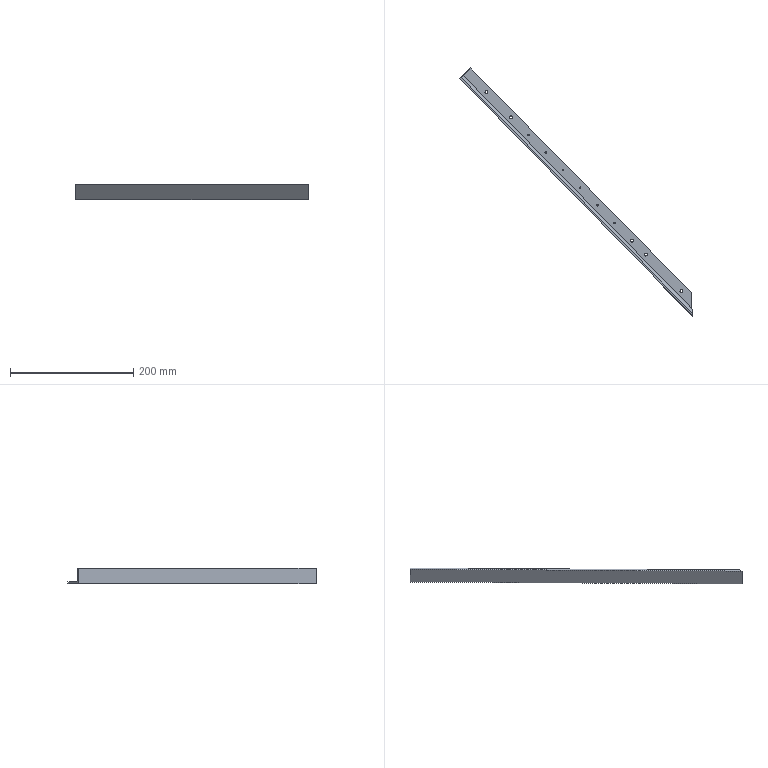Part | NX | features MG0301 nose pivot 24(right) 2 | 1 solid | 20 faces | box 376.796 x 401.943 x 25.4 mm | volume 82340 mm3 | cylinder 12 | plane 8 | commonest cylinder face diameters 2.4 x6 4.763 x5 9.525 x1
STEP:
#1=CARTESIAN_POINT('',(-216.606,-252.536,3.175));
#2=VERTEX_POINT('',#1);
#3=CARTESIAN_POINT('',(-217.446,-251.679,3.175));
#4=DIRECTION('',(0.,0.,1.));
#5=DIRECTION('',(0.7002,-0.7139,0.));
#6=AXIS2_PLACEMENT_3D('',#3,#4,#5);
#7=CIRCLE('',#6,1.2);
#8=EDGE_CURVE('',#2,#2,#7,.T.);
#9=ORIENTED_EDGE('',*,*,#8,.F.);
#10=EDGE_LOOP('',(#9));
#11=FACE_BOUND('',#10,.T.);
#12=CARTESIAN_POINT('',(-160.587,-309.649,3.175));
#13=VERTEX_POINT('',#12);
#14=CARTESIAN_POINT('',(-161.428,-308.792,3.175));
#15=DIRECTION('',(0.,0.,1.));
#16=DIRECTION('',(0.7002,-0.7139,0.));
#17=AXIS2_PLACEMENT_3D('',#14,#15,#16);
#18=CIRCLE('',#17,1.2);
#19=EDGE_CURVE('',#13,#13,#18,.T.);
#20=ORIENTED_EDGE('',*,*,#19,.F.);
#21=EDGE_LOOP('',(#20));
#22=FACE_BOUND('',#21,.T.);
#23=CARTESIAN_POINT('',(-104.569,-366.762,3.175));
#24=VERTEX_POINT('',#23);
#25=CARTESIAN_POINT('',(-105.409,-365.905,3.175));
#26=DIRECTION('',(0.,0.,1.));
#27=DIRECTION('',(0.7002,-0.7139,0.));
#28=AXIS2_PLACEMENT_3D('',#25,#26,#27);
#29=CIRCLE('',#28,1.2);
#30=EDGE_CURVE('',#24,#24,#29,.T.);
#31=ORIENTED_EDGE('',*,*,#30,.F.);
#32=EDGE_LOOP('',(#31));
#33=FACE_BOUND('',#32,.T.);
#34=CARTESIAN_POINT('',(-271.084,-194.566,3.175));
#35=VERTEX_POINT('',#34);
#36=CARTESIAN_POINT('',(-273.465,-194.566,3.175));
#37=DIRECTION('',(0.,0.,1.));
#38=DIRECTION('',(1.,0.,0.));
#39=AXIS2_PLACEMENT_3D('',#36,#37,#38);
#40=CIRCLE('',#39,2.381);
#41=EDGE_CURVE('',#35,#35,#40,.T.);
#42=ORIENTED_EDGE('',*,*,#41,.F.);
#43=EDGE_LOOP('',(#42));
#44=FACE_BOUND('',#43,.T.);
#45=CARTESIAN_POINT('',(-310.915,-153.957,3.175));
#46=VERTEX_POINT('',#45);
#47=CARTESIAN_POINT('',(-313.296,-153.957,3.175));
#48=DIRECTION('',(0.,0.,1.));
#49=DIRECTION('',(1.,0.,0.));
#50=AXIS2_PLACEMENT_3D('',#47,#48,#49);
#51=CIRCLE('',#50,2.381);
#52=EDGE_CURVE('',#46,#46,#51,.T.);
#53=ORIENTED_EDGE('',*,*,#52,.F.);
#54=EDGE_LOOP('',(#53));
#55=FACE_BOUND('',#54,.T.);
#56=CARTESIAN_POINT('',(-52.781,-417.134,3.175));
#57=VERTEX_POINT('',#56);
#58=CARTESIAN_POINT('',(-55.162,-417.134,3.175));
#59=DIRECTION('',(0.,0.,1.));
#60=DIRECTION('',(1.,0.,0.));
#61=AXIS2_PLACEMENT_3D('',#58,#59,#60);
#62=CIRCLE('',#61,2.381);
#63=EDGE_CURVE('',#57,#57,#62,.T.);
#64=ORIENTED_EDGE('',*,*,#63,.F.);
#65=EDGE_LOOP('',(#64));
#66=FACE_BOUND('',#65,.T.);
#67=CARTESIAN_POINT('',(-75.013,-394.467,3.175));
#68=VERTEX_POINT('',#67);
#69=CARTESIAN_POINT('',(-77.394,-394.467,3.175));
#70=DIRECTION('',(0.,0.,1.));
#71=DIRECTION('',(1.,0.,0.));
#72=AXIS2_PLACEMENT_3D('',#69,#70,#71);
#73=CIRCLE('',#72,2.381);
#74=EDGE_CURVE('',#68,#68,#73,.T.);
#75=ORIENTED_EDGE('',*,*,#74,.F.);
#76=EDGE_LOOP('',(#75));
#77=FACE_BOUND('',#76,.T.);
#78=CARTESIAN_POINT('',(5.15,-476.196,3.175));
#79=VERTEX_POINT('',#78);
#80=CARTESIAN_POINT('',(2.768,-476.196,3.175));
#81=DIRECTION('',(0.,0.,1.));
#82=DIRECTION('',(1.,0.,0.));
#83=AXIS2_PLACEMENT_3D('',#80,#81,#82);
#84=CIRCLE('',#83,2.381);
#85=EDGE_CURVE('',#79,#79,#84,.T.);
#86=ORIENTED_EDGE('',*,*,#85,.F.);
#87=EDGE_LOOP('',(#86));
#88=FACE_BOUND('',#87,.T.);
#89=CARTESIAN_POINT('',(-338.421,-114.738,3.175));
#90=VERTEX_POINT('',#89);
#91=CARTESIAN_POINT('',(18.761,-478.899,3.175));
#92=VERTEX_POINT('',#91);
#93=CARTESIAN_POINT('',(-338.421,-114.738,3.175));
#94=DIRECTION('',(0.7002,-0.7139,0.));
#95=VECTOR('',#94,1000.);
#96=LINE('',#93,#95);
#97=EDGE_CURVE('',#90,#92,#96,.T.);
#98=ORIENTED_EDGE('',*,*,#97,.F.);
#99=CARTESIAN_POINT('',(-350.888,-126.966,3.175));
#100=VERTEX_POINT('',#99);
#101=CARTESIAN_POINT('',(-338.421,-114.738,3.175));
#102=DIRECTION('',(-0.7139,-0.7002,0.));
#103=VECTOR('',#102,1000.);
#104=LINE('',#101,#103);
#105=EDGE_CURVE('',#90,#100,#104,.T.);
#106=ORIENTED_EDGE('',*,*,#105,.T.);
#107=CARTESIAN_POINT('',(19.779,-504.875,3.175));
#108=VERTEX_POINT('',#107);
#109=CARTESIAN_POINT('',(-350.888,-126.966,3.175));
#110=DIRECTION('',(0.7002,-0.7139,0.));
#111=VECTOR('',#110,1000.);
#112=LINE('',#109,#111);
#113=EDGE_CURVE('',#100,#108,#112,.T.);
#114=ORIENTED_EDGE('',*,*,#113,.T.);
#115=CARTESIAN_POINT('',(3.97,-101.325,3.175));
#116=DIRECTION('',(0.03915,-0.9992,0.));
#117=VECTOR('',#116,1000.);
#118=LINE('',#115,#117);
#119=EDGE_CURVE('',#92,#108,#118,.T.);
#120=ORIENTED_EDGE('',*,*,#119,.F.);
#121=EDGE_LOOP('',(#98,#106,#114,#120));
#122=FACE_BOUND('',#121,.T.);
#123=CARTESIAN_POINT('',(-132.578,-338.206,3.175));
#124=VERTEX_POINT('',#123);
#125=CARTESIAN_POINT('',(-133.418,-337.349,3.175));
#126=DIRECTION('',(0.,0.,1.));
#127=DIRECTION('',(0.7002,-0.7139,0.));
#128=AXIS2_PLACEMENT_3D('',#125,#126,#127);
#129=CIRCLE('',#128,1.2);
#130=EDGE_CURVE('',#124,#124,#129,.T.);
#131=ORIENTED_EDGE('',*,*,#130,.F.);
#132=EDGE_LOOP('',(#131));
#133=FACE_BOUND('',#132,.T.);
#134=CARTESIAN_POINT('',(-188.597,-281.092,3.175));
#135=VERTEX_POINT('',#134);
#136=CARTESIAN_POINT('',(-189.437,-280.236,3.175));
#137=DIRECTION('',(0.,0.,1.));
#138=DIRECTION('',(0.7002,-0.7139,0.));
#139=AXIS2_PLACEMENT_3D('',#136,#137,#138);
#140=CIRCLE('',#139,1.2);
#141=EDGE_CURVE('',#135,#135,#140,.T.);
#142=ORIENTED_EDGE('',*,*,#141,.F.);
#143=EDGE_LOOP('',(#142));
#144=FACE_BOUND('',#143,.T.);
#145=CARTESIAN_POINT('',(-244.615,-223.979,3.175));
#146=VERTEX_POINT('',#145);
#147=CARTESIAN_POINT('',(-245.456,-223.123,3.175));
#148=DIRECTION('',(0.,0.,1.));
#149=DIRECTION('',(0.7002,-0.7139,0.));
#150=AXIS2_PLACEMENT_3D('',#147,#148,#149);
#151=CIRCLE('',#150,1.2);
#152=EDGE_CURVE('',#146,#146,#151,.T.);
#153=ORIENTED_EDGE('',*,*,#152,.F.);
#154=EDGE_LOOP('',(#153));
#155=FACE_BOUND('',#154,.T.);
#156=CARTESIAN_POINT('',(-338.421,-114.738,3.175));
#157=DIRECTION('',(0.,0.,-1.));
#158=DIRECTION('',(1.,0.,0.));
#159=AXIS2_PLACEMENT_3D('',#156,#157,#158);
#160=PLANE('',#159);
#161=ADVANCED_FACE('',(#11,#22,#33,#44,#55,#66,#77,#88,#122,#133,#144,#155),#160,.F.);
#162=CARTESIAN_POINT('',(-356.555,-132.524,25.4));
#163=VERTEX_POINT('',#162);
#164=CARTESIAN_POINT('',(20.242,-516.682,25.4));
#165=VERTEX_POINT('',#164);
#166=CARTESIAN_POINT('',(-356.555,-132.524,25.4));
#167=DIRECTION('',(0.7002,-0.7139,0.));
#168=VECTOR('',#167,1000.);
#169=LINE('',#166,#168);
#170=EDGE_CURVE('',#163,#165,#169,.T.);
#171=ORIENTED_EDGE('',*,*,#170,.F.);
#172=CARTESIAN_POINT('',(-356.555,-132.524,0.));
#173=VERTEX_POINT('',#172);
#174=CARTESIAN_POINT('',(-356.555,-132.524,0.));
#175=DIRECTION('',(0.,0.,-1.));
#176=VECTOR('',#175,1000.);
#177=LINE('',#174,#176);
#178=EDGE_CURVE('',#163,#173,#177,.T.);
#179=ORIENTED_EDGE('',*,*,#178,.T.);
#180=CARTESIAN_POINT('',(20.242,-516.682,0.));
#181=VERTEX_POINT('',#180);
#182=CARTESIAN_POINT('',(-356.555,-132.524,0.));
#183=DIRECTION('',(0.7002,-0.7139,0.));
#184=VECTOR('',#183,1000.);
#185=LINE('',#182,#184);
#186=EDGE_CURVE('',#173,#181,#185,.T.);
#187=ORIENTED_EDGE('',*,*,#186,.T.);
#188=CARTESIAN_POINT('',(20.242,-516.682,0.));
#189=DIRECTION('',(0.,0.,-1.));
#190=VECTOR('',#189,1000.);
#191=LINE('',#188,#190);
#192=EDGE_CURVE('',#165,#181,#191,.T.);
#193=ORIENTED_EDGE('',*,*,#192,.F.);
#194=EDGE_LOOP('',(#171,#179,#187,#193));
#195=FACE_BOUND('',#194,.T.);
#196=CARTESIAN_POINT('',(-356.555,-132.524,0.));
#197=DIRECTION('',(0.7139,0.7002,0.));
#198=DIRECTION('',(-0.7002,0.7139,0.));
#199=AXIS2_PLACEMENT_3D('',#196,#197,#198);
#200=PLANE('',#199);
#201=ADVANCED_FACE('',(#195),#200,.F.);
#202=CARTESIAN_POINT('',(-244.256,-223.123,0.));
#203=VERTEX_POINT('',#202);
#204=CARTESIAN_POINT('',(-245.456,-223.123,0.));
#205=DIRECTION('',(0.,0.,1.));
#206=DIRECTION('',(1.,0.,0.));
#207=AXIS2_PLACEMENT_3D('',#204,#205,#206);
#208=CIRCLE('',#207,1.2);
#209=EDGE_CURVE('',#203,#203,#208,.T.);
#210=ORIENTED_EDGE('',*,*,#209,.T.);
#211=EDGE_LOOP('',(#210));
#212=FACE_BOUND('',#211,.T.);
#213=CARTESIAN_POINT('',(-216.246,-251.679,0.));
#214=VERTEX_POINT('',#213);
#215=CARTESIAN_POINT('',(-217.446,-251.679,0.));
#216=DIRECTION('',(0.,0.,1.));
#217=DIRECTION('',(1.,0.,0.));
#218=AXIS2_PLACEMENT_3D('',#215,#216,#217);
#219=CIRCLE('',#218,1.2);
#220=EDGE_CURVE('',#214,#214,#219,.T.);
#221=ORIENTED_EDGE('',*,*,#220,.T.);
#222=EDGE_LOOP('',(#221));
#223=FACE_BOUND('',#222,.T.);
#224=CARTESIAN_POINT('',(-188.237,-280.236,0.));
#225=VERTEX_POINT('',#224);
#226=CARTESIAN_POINT('',(-189.437,-280.236,0.));
#227=DIRECTION('',(0.,0.,1.));
#228=DIRECTION('',(1.,0.,0.));
#229=AXIS2_PLACEMENT_3D('',#226,#227,#228);
#230=CIRCLE('',#229,1.2);
#231=EDGE_CURVE('',#225,#225,#230,.T.);
#232=ORIENTED_EDGE('',*,*,#231,.T.);
#233=EDGE_LOOP('',(#232));
#234=FACE_BOUND('',#233,.T.);
#235=CARTESIAN_POINT('',(-160.228,-308.792,0.));
#236=VERTEX_POINT('',#235);
#237=CARTESIAN_POINT('',(-161.428,-308.792,0.));
#238=DIRECTION('',(0.,0.,1.));
#239=DIRECTION('',(1.,0.,0.));
#240=AXIS2_PLACEMENT_3D('',#237,#238,#239);
#241=CIRCLE('',#240,1.2);
#242=EDGE_CURVE('',#236,#236,#241,.T.);
#243=ORIENTED_EDGE('',*,*,#242,.T.);
#244=EDGE_LOOP('',(#243));
#245=FACE_BOUND('',#244,.T.);
#246=CARTESIAN_POINT('',(-132.218,-337.349,0.));
#247=VERTEX_POINT('',#246);
#248=CARTESIAN_POINT('',(-133.418,-337.349,0.));
#249=DIRECTION('',(0.,0.,1.));
#250=DIRECTION('',(1.,0.,0.));
#251=AXIS2_PLACEMENT_3D('',#248,#249,#250);
#252=CIRCLE('',#251,1.2);
#253=EDGE_CURVE('',#247,#247,#252,.T.);
#254=ORIENTED_EDGE('',*,*,#253,.T.);
#255=EDGE_LOOP('',(#254));
#256=FACE_BOUND('',#255,.T.);
#257=CARTESIAN_POINT('',(-104.209,-365.905,0.));
#258=VERTEX_POINT('',#257);
#259=CARTESIAN_POINT('',(-105.409,-365.905,0.));
#260=DIRECTION('',(0.,0.,1.));
#261=DIRECTION('',(1.,0.,0.));
#262=AXIS2_PLACEMENT_3D('',#259,#260,#261);
#263=CIRCLE('',#262,1.2);
#264=EDGE_CURVE('',#258,#258,#263,.T.);
#265=ORIENTED_EDGE('',*,*,#264,.T.);
#266=EDGE_LOOP('',(#265));
#267=FACE_BOUND('',#266,.T.);
#268=CARTESIAN_POINT('',(-271.084,-194.566,0.));
#269=VERTEX_POINT('',#268);
#270=CARTESIAN_POINT('',(-273.465,-194.566,0.));
#271=DIRECTION('',(0.,0.,1.));
#272=DIRECTION('',(1.,0.,0.));
#273=AXIS2_PLACEMENT_3D('',#270,#271,#272);
#274=CIRCLE('',#273,2.381);
#275=EDGE_CURVE('',#269,#269,#274,.T.);
#276=ORIENTED_EDGE('',*,*,#275,.T.);
#277=EDGE_LOOP('',(#276));
#278=FACE_BOUND('',#277,.T.);
#279=CARTESIAN_POINT('',(-310.915,-153.957,0.));
#280=VERTEX_POINT('',#279);
#281=CARTESIAN_POINT('',(-313.296,-153.957,0.));
#282=DIRECTION('',(0.,0.,1.));
#283=DIRECTION('',(1.,0.,0.));
#284=AXIS2_PLACEMENT_3D('',#281,#282,#283);
#285=CIRCLE('',#284,2.381);
#286=EDGE_CURVE('',#280,#280,#285,.T.);
#287=ORIENTED_EDGE('',*,*,#286,.T.);
#288=EDGE_LOOP('',(#287));
#289=FACE_BOUND('',#288,.T.);
#290=CARTESIAN_POINT('',(-52.781,-417.134,0.));
#291=VERTEX_POINT('',#290);
#292=CARTESIAN_POINT('',(-55.162,-417.134,0.));
#293=DIRECTION('',(0.,0.,1.));
#294=DIRECTION('',(1.,0.,0.));
#295=AXIS2_PLACEMENT_3D('',#292,#293,#294);
#296=CIRCLE('',#295,2.381);
#297=EDGE_CURVE('',#291,#291,#296,.T.);
#298=ORIENTED_EDGE('',*,*,#297,.T.);
#299=EDGE_LOOP('',(#298));
#300=FACE_BOUND('',#299,.T.);
#301=CARTESIAN_POINT('',(-75.013,-394.467,0.));
#302=VERTEX_POINT('',#301);
#303=CARTESIAN_POINT('',(-77.394,-394.467,0.));
#304=DIRECTION('',(0.,0.,1.));
#305=DIRECTION('',(1.,0.,0.));
#306=AXIS2_PLACEMENT_3D('',#303,#304,#305);
#307=CIRCLE('',#306,2.381);
#308=EDGE_CURVE('',#302,#302,#307,.T.);
#309=ORIENTED_EDGE('',*,*,#308,.T.);
#310=EDGE_LOOP('',(#309));
#311=FACE_BOUND('',#310,.T.);
#312=CARTESIAN_POINT('',(5.15,-476.196,0.));
#313=VERTEX_POINT('',#312);
#314=CARTESIAN_POINT('',(2.768,-476.196,0.));
#315=DIRECTION('',(0.,0.,1.));
#316=DIRECTION('',(1.,0.,0.));
#317=AXIS2_PLACEMENT_3D('',#314,#315,#316);
#318=CIRCLE('',#317,2.381);
#319=EDGE_CURVE('',#313,#313,#318,.T.);
#320=ORIENTED_EDGE('',*,*,#319,.T.);
#321=EDGE_LOOP('',(#320));
#322=FACE_BOUND('',#321,.T.);
#323=ORIENTED_EDGE('',*,*,#186,.F.);
#324=CARTESIAN_POINT('',(-338.421,-114.738,0.));
#325=VERTEX_POINT('',#324);
#326=CARTESIAN_POINT('',(-356.555,-132.524,0.));
#327=DIRECTION('',(0.7139,0.7002,0.));
#328=VECTOR('',#327,1000.);
#329=LINE('',#326,#328);
#330=EDGE_CURVE('',#173,#325,#329,.T.);
#331=ORIENTED_EDGE('',*,*,#330,.T.);
#332=CARTESIAN_POINT('',(18.761,-478.899,0.));
#333=VERTEX_POINT('',#332);
#334=CARTESIAN_POINT('',(-338.421,-114.738,0.));
#335=DIRECTION('',(0.7002,-0.7139,0.));
#336=VECTOR('',#335,1000.);
#337=LINE('',#334,#336);
#338=EDGE_CURVE('',#325,#333,#337,.T.);
#339=ORIENTED_EDGE('',*,*,#338,.T.);
#340=CARTESIAN_POINT('',(4.637,-118.374,0.));
#341=DIRECTION('',(-0.03915,0.9992,0.));
#342=VECTOR('',#341,1000.);
#343=LINE('',#340,#342);
#344=EDGE_CURVE('',#181,#333,#343,.T.);
#345=ORIENTED_EDGE('',*,*,#344,.F.);
#346=EDGE_LOOP('',(#323,#331,#339,#345));
#347=FACE_BOUND('',#346,.T.);
#348=CARTESIAN_POINT('',(-356.555,-132.524,0.));
#349=DIRECTION('',(0.,0.,1.));
#350=DIRECTION('',(-1.,0.,0.));
#351=AXIS2_PLACEMENT_3D('',#348,#349,#350);
#352=PLANE('',#351);
#353=ADVANCED_FACE('',(#212,#223,#234,#245,#256,#267,#278,#289,#300,#311,#322,#347),#352,.F.);
#354=ORIENTED_EDGE('',*,*,#338,.F.);
#355=CARTESIAN_POINT('',(-338.421,-114.738,0.));
#356=DIRECTION('',(0.,0.,1.));
#357=VECTOR('',#356,1000.);
#358=LINE('',#355,#357);
#359=EDGE_CURVE('',#325,#90,#358,.T.);
#360=ORIENTED_EDGE('',*,*,#359,.T.);
#361=ORIENTED_EDGE('',*,*,#97,.T.);
#362=CARTESIAN_POINT('',(18.761,-478.899,0.));
#363=DIRECTION('',(0.,0.,1.));
#364=VECTOR('',#363,1000.);
#365=LINE('',#362,#364);
#366=EDGE_CURVE('',#333,#92,#365,.T.);
#367=ORIENTED_EDGE('',*,*,#366,.F.);
#368=EDGE_LOOP('',(#354,#360,#361,#367));
#369=FACE_BOUND('',#368,.T.);
#370=CARTESIAN_POINT('',(-338.421,-114.738,0.));
#371=DIRECTION('',(-0.7139,-0.7002,0.));
#372=DIRECTION('',(0.7002,-0.7139,0.));
#373=AXIS2_PLACEMENT_3D('',#370,#371,#372);
#374=PLANE('',#373);
#375=ADVANCED_FACE('',(#369),#374,.F.);
#376=ORIENTED_EDGE('',*,*,#113,.F.);
#377=CARTESIAN_POINT('',(-354.288,-130.301,7.938));
#378=VERTEX_POINT('',#377);
#379=CARTESIAN_POINT('',(-350.888,-126.966,7.938));
#380=DIRECTION('',(-0.7002,0.7139,0.));
#381=DIRECTION('',(-0.7139,-0.7002,0.));
#382=AXIS2_PLACEMENT_3D('',#379,#380,#381);
#383=CIRCLE('',#382,4.763);
#384=EDGE_CURVE('',#100,#378,#383,.T.);
#385=ORIENTED_EDGE('',*,*,#384,.T.);
#386=CARTESIAN_POINT('',(20.057,-511.959,7.938));
#387=VERTEX_POINT('',#386);
#388=CARTESIAN_POINT('',(-354.288,-130.301,7.938));
#389=DIRECTION('',(0.7002,-0.7139,0.));
#390=VECTOR('',#389,1000.);
#391=LINE('',#388,#390);
#392=EDGE_CURVE('',#378,#387,#391,.T.);
#393=ORIENTED_EDGE('',*,*,#392,.T.);
#394=CARTESIAN_POINT('',(19.779,-504.875,7.938));
#395=DIRECTION('',(0.9992,0.03915,0.));
#396=DIRECTION('',(0.03915,-0.9992,0.));
#397=AXIS2_PLACEMENT_3D('',#394,#395,#396);
#398=ELLIPSE('',#397,7.09,4.763);
#399=EDGE_CURVE('',#108,#387,#398,.F.);
#400=ORIENTED_EDGE('',*,*,#399,.F.);
#401=EDGE_LOOP('',(#376,#385,#393,#400));
#402=FACE_BOUND('',#401,.T.);
#403=CARTESIAN_POINT('',(-350.888,-126.966,7.938));
#404=DIRECTION('',(0.7002,-0.7139,0.));
#405=DIRECTION('',(0.7139,0.7002,0.));
#406=AXIS2_PLACEMENT_3D('',#403,#404,#405);
#407=CYLINDRICAL_SURFACE('',#406,4.763);
#408=ADVANCED_FACE('',(#402),#407,.F.);
#409=ORIENTED_EDGE('',*,*,#392,.F.);
#410=CARTESIAN_POINT('',(-354.288,-130.301,25.4));
#411=VERTEX_POINT('',#410);
#412=CARTESIAN_POINT('',(-354.288,-130.301,25.4));
#413=DIRECTION('',(0.,0.,1.));
#414=VECTOR('',#413,1000.);
#415=LINE('',#412,#414);
#416=EDGE_CURVE('',#378,#411,#415,.T.);
#417=ORIENTED_EDGE('',*,*,#416,.T.);
#418=CARTESIAN_POINT('',(20.057,-511.959,25.4));
#419=VERTEX_POINT('',#418);
#420=CARTESIAN_POINT('',(-354.288,-130.301,25.4));
#421=DIRECTION('',(0.7002,-0.7139,0.));
#422=VECTOR('',#421,1000.);
#423=LINE('',#420,#422);
#424=EDGE_CURVE('',#411,#419,#423,.T.);
#425=ORIENTED_EDGE('',*,*,#424,.T.);
#426=CARTESIAN_POINT('',(20.057,-511.959,25.4));
#427=DIRECTION('',(0.,0.,1.));
#428=VECTOR('',#427,1000.);
#429=LINE('',#426,#428);
#430=EDGE_CURVE('',#387,#419,#429,.T.);
#431=ORIENTED_EDGE('',*,*,#430,.F.);
#432=EDGE_LOOP('',(#409,#417,#425,#431));
#433=FACE_BOUND('',#432,.T.);
#434=CARTESIAN_POINT('',(-354.288,-130.301,25.4));
#435=DIRECTION('',(-0.7139,-0.7002,0.));
#436=DIRECTION('',(0.7002,-0.7139,0.));
#437=AXIS2_PLACEMENT_3D('',#434,#435,#436);
#438=PLANE('',#437);
#439=ADVANCED_FACE('',(#433),#438,.F.);
#440=ORIENTED_EDGE('',*,*,#424,.F.);
#441=CARTESIAN_POINT('',(-356.555,-132.524,25.4));
#442=DIRECTION('',(-0.7139,-0.7002,0.));
#443=VECTOR('',#442,1000.);
#444=LINE('',#441,#443);
#445=EDGE_CURVE('',#411,#163,#444,.T.);
#446=ORIENTED_EDGE('',*,*,#445,.T.);
#447=ORIENTED_EDGE('',*,*,#170,.T.);
#448=CARTESIAN_POINT('',(4.637,-118.374,25.4));
#449=DIRECTION('',(0.03915,-0.9992,0.));
#450=VECTOR('',#449,1000.);
#451=LINE('',#448,#450);
#452=EDGE_CURVE('',#419,#165,#451,.T.);
#453=ORIENTED_EDGE('',*,*,#452,.F.);
#454=EDGE_LOOP('',(#440,#446,#447,#453));
#455=FACE_BOUND('',#454,.T.);
#456=CARTESIAN_POINT('',(-356.555,-132.524,25.4));
#457=DIRECTION('',(0.,0.,-1.));
#458=DIRECTION('',(1.,0.,0.));
#459=AXIS2_PLACEMENT_3D('',#456,#457,#458);
#460=PLANE('',#459);
#461=ADVANCED_FACE('',(#455),#460,.F.);
#462=ORIENTED_EDGE('',*,*,#178,.F.);
#463=ORIENTED_EDGE('',*,*,#445,.F.);
#464=ORIENTED_EDGE('',*,*,#416,.F.);
#465=ORIENTED_EDGE('',*,*,#384,.F.);
#466=ORIENTED_EDGE('',*,*,#105,.F.);
#467=ORIENTED_EDGE('',*,*,#359,.F.);
#468=ORIENTED_EDGE('',*,*,#330,.F.);
#469=EDGE_LOOP('',(#462,#463,#464,#465,#466,#467,#468));
#470=FACE_BOUND('',#469,.T.);
#471=CARTESIAN_POINT('',(-350.888,-126.966,7.938));
#472=DIRECTION('',(-0.7002,0.7139,0.));
#473=DIRECTION('',(-0.7139,-0.7002,0.));
#474=AXIS2_PLACEMENT_3D('',#471,#472,#473);
#475=PLANE('',#474);
#476=ADVANCED_FACE('',(#470),#475,.T.);
#477=ORIENTED_EDGE('',*,*,#344,.T.);
#478=ORIENTED_EDGE('',*,*,#366,.T.);
#479=ORIENTED_EDGE('',*,*,#119,.T.);
#480=ORIENTED_EDGE('',*,*,#399,.T.);
#481=ORIENTED_EDGE('',*,*,#430,.T.);
#482=ORIENTED_EDGE('',*,*,#452,.T.);
#483=ORIENTED_EDGE('',*,*,#192,.T.);
#484=EDGE_LOOP('',(#477,#478,#479,#480,#481,#482,#483));
#485=FACE_BOUND('',#484,.T.);
#486=CARTESIAN_POINT('',(20.242,-516.682,-856.077));
#487=DIRECTION('',(-0.9992,-0.03915,0.));
#488=DIRECTION('',(0.03915,-0.9992,0.));
#489=AXIS2_PLACEMENT_3D('',#486,#487,#488);
#490=PLANE('',#489);
#491=ADVANCED_FACE('',(#485),#490,.F.);
#492=ORIENTED_EDGE('',*,*,#319,.F.);
#493=EDGE_LOOP('',(#492));
#494=FACE_BOUND('',#493,.T.);
#495=ORIENTED_EDGE('',*,*,#85,.T.);
#496=EDGE_LOOP('',(#495));
#497=FACE_BOUND('',#496,.T.);
#498=CARTESIAN_POINT('',(2.768,-476.196,63.5));
#499=DIRECTION('',(0.,0.,-1.));
#500=DIRECTION('',(1.,0.,0.));
#501=AXIS2_PLACEMENT_3D('',#498,#499,#500);
#502=CYLINDRICAL_SURFACE('',#501,2.381);
#503=ADVANCED_FACE('',(#494,#497),#502,.F.);
#504=ORIENTED_EDGE('',*,*,#308,.F.);
#505=EDGE_LOOP('',(#504));
#506=FACE_BOUND('',#505,.T.);
#507=ORIENTED_EDGE('',*,*,#74,.T.);
#508=EDGE_LOOP('',(#507));
#509=FACE_BOUND('',#508,.T.);
#510=CARTESIAN_POINT('',(-77.394,-394.467,63.5));
#511=DIRECTION('',(0.,0.,-1.));
#512=DIRECTION('',(1.,0.,0.));
#513=AXIS2_PLACEMENT_3D('',#510,#511,#512);
#514=CYLINDRICAL_SURFACE('',#513,2.381);
#515=ADVANCED_FACE('',(#506,#509),#514,.F.);
#516=ORIENTED_EDGE('',*,*,#297,.F.);
#517=EDGE_LOOP('',(#516));
#518=FACE_BOUND('',#517,.T.);
#519=ORIENTED_EDGE('',*,*,#63,.T.);
#520=EDGE_LOOP('',(#519));
#521=FACE_BOUND('',#520,.T.);
#522=CARTESIAN_POINT('',(-55.162,-417.134,63.5));
#523=DIRECTION('',(0.,0.,-1.));
#524=DIRECTION('',(1.,0.,0.));
#525=AXIS2_PLACEMENT_3D('',#522,#523,#524);
#526=CYLINDRICAL_SURFACE('',#525,2.381);
#527=ADVANCED_FACE('',(#518,#521),#526,.F.);
#528=ORIENTED_EDGE('',*,*,#286,.F.);
#529=EDGE_LOOP('',(#528));
#530=FACE_BOUND('',#529,.T.);
#531=ORIENTED_EDGE('',*,*,#52,.T.);
#532=EDGE_LOOP('',(#531));
#533=FACE_BOUND('',#532,.T.);
#534=CARTESIAN_POINT('',(-313.296,-153.957,63.5));
#535=DIRECTION('',(0.,0.,-1.));
#536=DIRECTION('',(1.,0.,0.));
#537=AXIS2_PLACEMENT_3D('',#534,#535,#536);
#538=CYLINDRICAL_SURFACE('',#537,2.381);
#539=ADVANCED_FACE('',(#530,#533),#538,.F.);
#540=ORIENTED_EDGE('',*,*,#275,.F.);
#541=EDGE_LOOP('',(#540));
#542=FACE_BOUND('',#541,.T.);
#543=ORIENTED_EDGE('',*,*,#41,.T.);
#544=EDGE_LOOP('',(#543));
#545=FACE_BOUND('',#544,.T.);
#546=CARTESIAN_POINT('',(-273.465,-194.566,63.5));
#547=DIRECTION('',(0.,0.,-1.));
#548=DIRECTION('',(1.,0.,0.));
#549=AXIS2_PLACEMENT_3D('',#546,#547,#548);
#550=CYLINDRICAL_SURFACE('',#549,2.381);
#551=ADVANCED_FACE('',(#542,#545),#550,.F.);
#552=ORIENTED_EDGE('',*,*,#30,.T.);
#553=EDGE_LOOP('',(#552));
#554=FACE_BOUND('',#553,.T.);
#555=ORIENTED_EDGE('',*,*,#264,.F.);
#556=EDGE_LOOP('',(#555));
#557=FACE_BOUND('',#556,.T.);
#558=CARTESIAN_POINT('',(-105.409,-365.905,-6.825));
#559=DIRECTION('',(0.,0.,1.));
#560=DIRECTION('',(1.,0.,0.));
#561=AXIS2_PLACEMENT_3D('',#558,#559,#560);
#562=CYLINDRICAL_SURFACE('',#561,1.2);
#563=ADVANCED_FACE('',(#554,#557),#562,.F.);
#564=ORIENTED_EDGE('',*,*,#130,.T.);
#565=EDGE_LOOP('',(#564));
#566=FACE_BOUND('',#565,.T.);
#567=ORIENTED_EDGE('',*,*,#253,.F.);
#568=EDGE_LOOP('',(#567));
#569=FACE_BOUND('',#568,.T.);
#570=CARTESIAN_POINT('',(-133.418,-337.349,-6.825));
#571=DIRECTION('',(0.,0.,1.));
#572=DIRECTION('',(1.,0.,0.));
#573=AXIS2_PLACEMENT_3D('',#570,#571,#572);
#574=CYLINDRICAL_SURFACE('',#573,1.2);
#575=ADVANCED_FACE('',(#566,#569),#574,.F.);
#576=ORIENTED_EDGE('',*,*,#19,.T.);
#577=EDGE_LOOP('',(#576));
#578=FACE_BOUND('',#577,.T.);
#579=ORIENTED_EDGE('',*,*,#242,.F.);
#580=EDGE_LOOP('',(#579));
#581=FACE_BOUND('',#580,.T.);
#582=CARTESIAN_POINT('',(-161.428,-308.792,-6.825));
#583=DIRECTION('',(0.,0.,1.));
#584=DIRECTION('',(1.,0.,0.));
#585=AXIS2_PLACEMENT_3D('',#582,#583,#584);
#586=CYLINDRICAL_SURFACE('',#585,1.2);
#587=ADVANCED_FACE('',(#578,#581),#586,.F.);
#588=ORIENTED_EDGE('',*,*,#141,.T.);
#589=EDGE_LOOP('',(#588));
#590=FACE_BOUND('',#589,.T.);
#591=ORIENTED_EDGE('',*,*,#231,.F.);
#592=EDGE_LOOP('',(#591));
#593=FACE_BOUND('',#592,.T.);
#594=CARTESIAN_POINT('',(-189.437,-280.236,-6.825));
#595=DIRECTION('',(0.,0.,1.));
#596=DIRECTION('',(1.,0.,0.));
#597=AXIS2_PLACEMENT_3D('',#594,#595,#596);
#598=CYLINDRICAL_SURFACE('',#597,1.2);
#599=ADVANCED_FACE('',(#590,#593),#598,.F.);
#600=ORIENTED_EDGE('',*,*,#8,.T.);
#601=EDGE_LOOP('',(#600));
#602=FACE_BOUND('',#601,.T.);
#603=ORIENTED_EDGE('',*,*,#220,.F.);
#604=EDGE_LOOP('',(#603));
#605=FACE_BOUND('',#604,.T.);
#606=CARTESIAN_POINT('',(-217.446,-251.679,-6.825));
#607=DIRECTION('',(0.,0.,1.));
#608=DIRECTION('',(1.,0.,0.));
#609=AXIS2_PLACEMENT_3D('',#606,#607,#608);
#610=CYLINDRICAL_SURFACE('',#609,1.2);
#611=ADVANCED_FACE('',(#602,#605),#610,.F.);
#612=ORIENTED_EDGE('',*,*,#152,.T.);
#613=EDGE_LOOP('',(#612));
#614=FACE_BOUND('',#613,.T.);
#615=ORIENTED_EDGE('',*,*,#209,.F.);
#616=EDGE_LOOP('',(#615));
#617=FACE_BOUND('',#616,.T.);
#618=CARTESIAN_POINT('',(-245.456,-223.123,-6.825));
#619=DIRECTION('',(0.,0.,1.));
#620=DIRECTION('',(1.,0.,0.));
#621=AXIS2_PLACEMENT_3D('',#618,#619,#620);
#622=CYLINDRICAL_SURFACE('',#621,1.2);
#623=ADVANCED_FACE('',(#614,#617),#622,.F.);
#624=CLOSED_SHELL('',(#161,#201,#353,#375,#408,#439,#461,#476,#491,#503,#515,#527,#539,#551,#563,#575,#587,#599,#611,#623));
#625=MANIFOLD_SOLID_BREP('',#624);
#626=(LENGTH_UNIT()NAMED_UNIT(*)SI_UNIT(.MILLI.,.METRE.));
#627=UNCERTAINTY_MEASURE_WITH_UNIT(LENGTH_MEASURE(0.00001),#626,'','');
#628=(NAMED_UNIT(*)PLANE_ANGLE_UNIT()SI_UNIT($,.RADIAN.));
#629=(NAMED_UNIT(*)SI_UNIT($,.STERADIAN.)SOLID_ANGLE_UNIT());
#630=(GEOMETRIC_REPRESENTATION_CONTEXT(3)GLOBAL_UNCERTAINTY_ASSIGNED_CONTEXT((#627))GLOBAL_UNIT_ASSIGNED_CONTEXT((#626,#628,#629))REPRESENTATION_CONTEXT('',''));
#631=ADVANCED_BREP_SHAPE_REPRESENTATION('',(#625),#630);